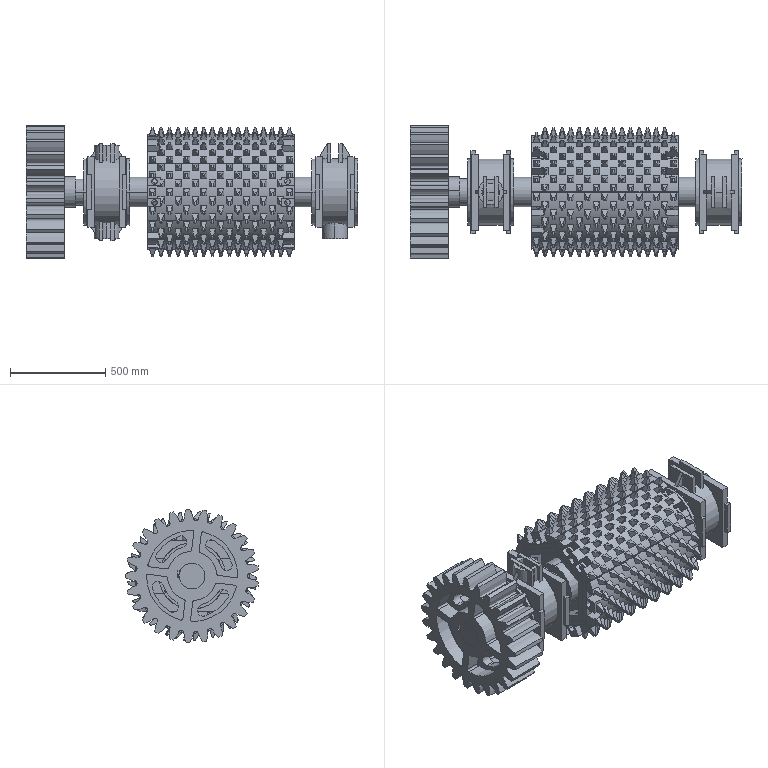Part | NX | features BREP 13, DATUM_CSYS 1, MOVE_FACE 1, SKETCH 1 | 26 solids | 4573 faces | volume 260357550 mm3 | plane 2966 | cylinder 1129 | cone 394 | spline 50 | torus 34 | commonest cylinder face diameters 38 x345 30 x96 20 x88 16 x72 10 x48 18 x48